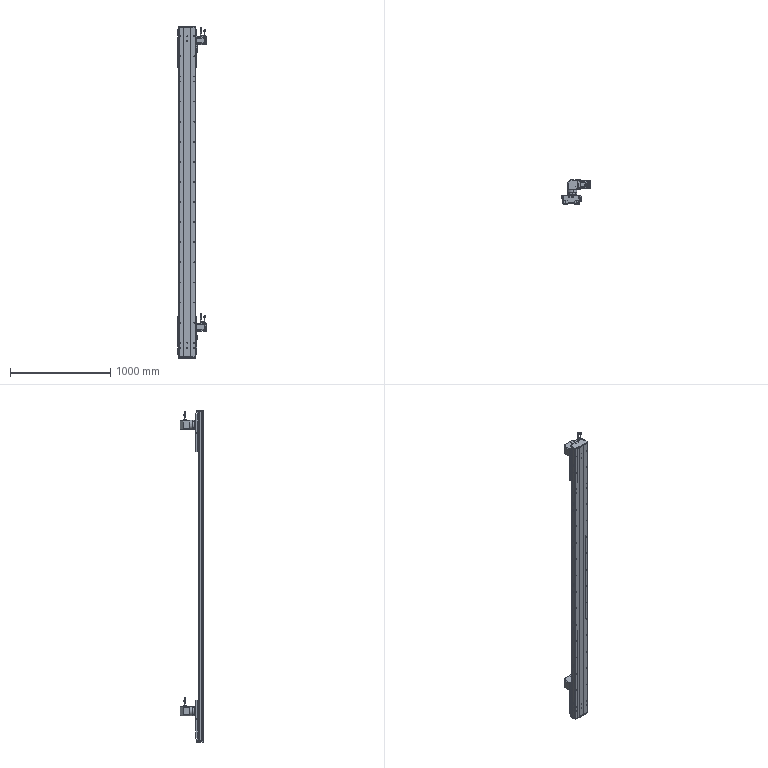Part | STEP file | EH17B-L13-C-S3000-ZP75-D3-N10 | 58 solids | 4152 faces | volume 18933367 mm3 | plane 2032 | cylinder 1599 | cone 241 | spline 224 | torus 56 | commonest cylinder face diameters 8 x72 8.6 x72 14 x72 1 x69 6 x67 5 x62